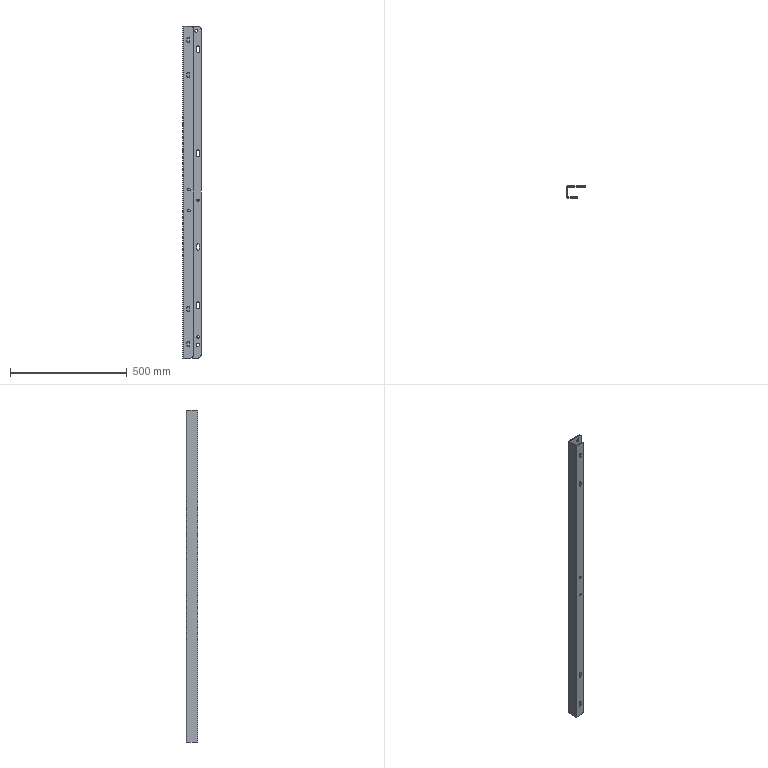Part | SolidWorks | features ICE 4, Cut 1, Fillet 1, FlatPattern 1, SMBaseFlange 1, SheetMetal 1 | 1 solid | 76 faces | box 77 x 50 x 1420 mm | volume 692252 mm3 | cylinder 40 | plane 36 | commonest cylinder face diameters 10 x12 12 x12 11 x6 24 x4 0.4 x2 6.4 x2